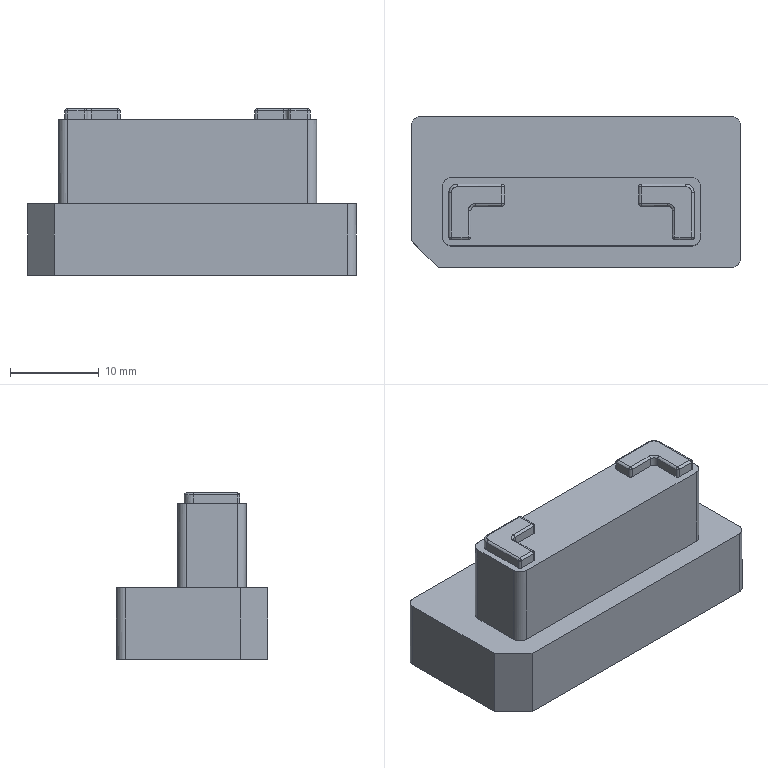CAM job | PowerMill | 3-axis milling, other | part box 37 x 17 x 18.689 mm
Tools:
number,name,type,diameter,tip_radius,length,cutting_length,overhang,flutes,holder,toolpaths_using
1,D10C,end_mill,10.0,0.0,60.0,,30.0,1,D42L35,1
2,D4C_1,end_mill,4.0,0.0,30.0,,4.0,1,D42L35,1
10,D3_1,end_mill,3.0,0.0,30.0,,3.0,1,D42L35,2
1,D10C_1_1_1,end_mill,10.0,0.0,60.0,,19.16,1,D42L35,3
3,D10_1_1_1,end_mill,10.0,0.0,60.0,,18.84,1,D42L35,4
8,D1_1_1,end_mill,1.0,0.0,3.0,,1.48,1,D42L35,1
13,Text_D4_1_1,taper_spherical,4.0,0.3,60.0,,10.96,1,D42L35,1
Operations:
program,toolpath,strategy,tool,tool_number,tool_diameter,tip_radius,flutes,spindle_rpm,feed_cut,surface_speed_m_min_computed,feed_per_tooth_computed,tolerance,thickness,stepover,stepdown,cut_length,cut_time_min,total_time_min,workplane
13-B01-1-F,精公开粗01-扫面平行-D10C,raster_area_clear,D10C_1_1_1,1,10.0,0.0,1.0,8000.0,10000.0,251.33,1.25,0.03,0.28,6.0,1.0,235.36,0.024,0.0295,
13-B01-1-F,精公开粗01-外形偏置-D10C,offset_area_clear,D10C_1_1_1,1,10.0,0.0,1.0,8000.0,10000.0,251.33,1.25,0.03,0.28,6.0,1.0,6754.269,0.675,0.7443,
13-B01-1-F,精公开粗01-基准台等高-D10C,constantz,D10C_1_1_1,1,10.0,0.0,1.0,8000.0,10000.0,251.33,1.25,0.03,0.07,5.0,0.4,3009.062,0.301,0.3106,
13-B01-1-F,精公再粗02-外形偏置-D4C,offset_area_clear,D4C_1,2,4.0,0.0,1.0,18000.0,6000.0,226.19,0.3333,0.03,0.0,2.0,1.0,438.204,0.073,0.1093,
13-B01-1-F,精公基准台01-平坦面平行-D10,raster_area_clear,D10_1_1_1,3,10.0,0.0,1.0,8500.0,600.0,267.04,0.0706,0.005,0.38,5.0,1.0,319.771,0.533,0.621,
13-B01-1-F,精公基准台01-基准面偏置-D10,offset_area_clear,D10_1_1_1,3,10.0,0.0,1.0,8500.0,600.0,267.04,0.0706,0.005,0.38,5.0,1.0,116.337,0.194,0.2131,
13-B01-1-F,精公基准台01-外形侧光-D10,profile_area_clear,D10_1_1_1,3,10.0,0.0,1.0,8500.0,600.0,267.04,0.0706,0.005,-0.07,0.08,1.0,205.868,0.343,0.364,
13-B01-1-F,精公基准台01-基准台侧光-D10,profile_area_clear,D10_1_1_1,3,10.0,0.0,1.0,8500.0,600.0,267.04,0.0706,0.005,0.0,0.08,1.0,273.233,0.455,0.5197,
13-B01-1-F,精公精光01-等高-D3,constantz,D3_1,10,3.0,0.0,1.0,18000.0,2000.0,169.65,0.1111,0.005,-0.075,5.0,0.02,2771.167,1.386,1.499,
13-B01-1-F,精公精光01-平坦面平行-D3,raster_area_clear,D3_1,10,3.0,0.0,1.0,18000.0,600.0,169.65,0.0333,0.005,0.375,1.5,1.0,117.886,0.197,0.2152,
13-B01-1-F,精公精光02-等高-D1,constantz,D1_1_1,8,1.0,0.0,1.0,20000.0,1000.0,62.83,0.05,0.005,-0.075,5.0,0.02,464.837,0.465,0.5372,
13-B01-1-F,精公刻字01-刻字-Text_D4,pattern,Text_D4_1_1,13,4.0,0.3,1.0,15000.0,1000.0,188.5,0.0667,0.005,0.0,5.0,1.0,55.255,0.055,0.0737,
,精公开粗01-外形偏置-D10C_Reference,offset_area_clear,D10C,1,10.0,0.0,1.0,8000.0,10000.0,251.33,1.25,0.03,0.28,6.0,1.0,13508.146,1.351,1.484,